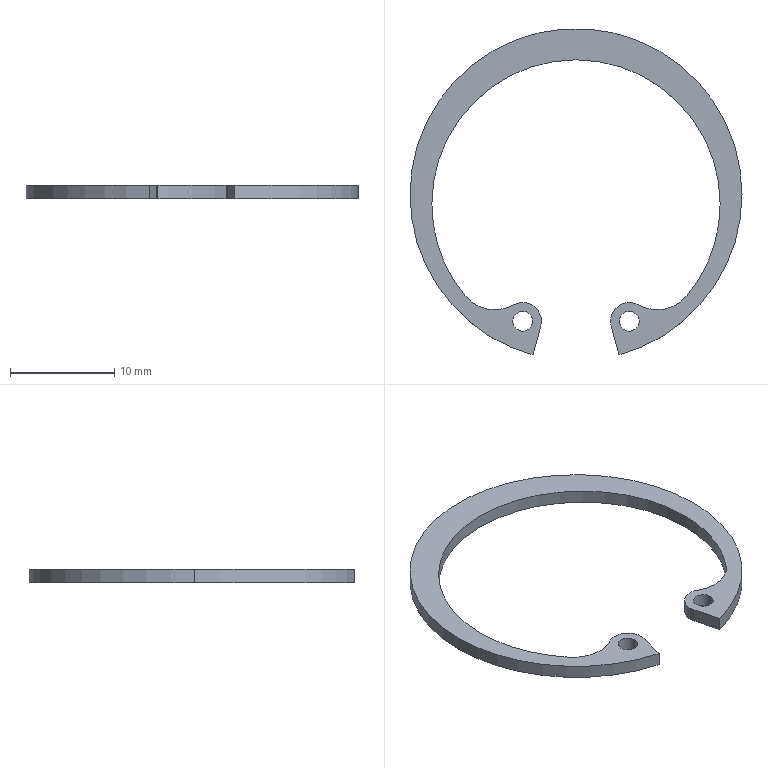Part | SolidWorks | features Extrusion 1 | 1 solid | 19 faces | box 31.9 x 31.357 x 1.3 mm | volume 270.021 mm3 | cylinder 15 | plane 4 | commonest cylinder face diameters 1.9 x4 3.6 x3 27.7 x3 31.9 x3 7.4 x2
STEP:
#1=CARTESIAN_POINT('',(-4.173,-11.265,1.3));
#2=VERTEX_POINT('',#1);
#3=CARTESIAN_POINT('',(-6.073,-11.265,1.3));
#4=VERTEX_POINT('',#3);
#5=CARTESIAN_POINT('',(-5.123,-11.265,1.3));
#6=DIRECTION('',(0.,0.,-1.));
#7=DIRECTION('',(1.,0.,0.));
#8=AXIS2_PLACEMENT_3D('',#5,#6,#7);
#9=CIRCLE('',#8,0.95);
#10=EDGE_CURVE('',#2,#4,#9,.T.);
#11=ORIENTED_EDGE('',*,*,#10,.F.);
#12=CARTESIAN_POINT('',(-4.173,-11.265,0.));
#13=VERTEX_POINT('',#12);
#14=CARTESIAN_POINT('',(-4.173,-11.265,1.3));
#15=DIRECTION('',(0.,0.,-1.));
#16=VECTOR('',#15,1000.);
#17=LINE('',#14,#16);
#18=EDGE_CURVE('',#2,#13,#17,.T.);
#19=ORIENTED_EDGE('',*,*,#18,.T.);
#20=CARTESIAN_POINT('',(-6.073,-11.265,0.));
#21=VERTEX_POINT('',#20);
#22=CARTESIAN_POINT('',(-5.123,-11.265,0.));
#23=DIRECTION('',(0.,0.,-1.));
#24=DIRECTION('',(1.,0.,0.));
#25=AXIS2_PLACEMENT_3D('',#22,#23,#24);
#26=CIRCLE('',#25,0.95);
#27=EDGE_CURVE('',#13,#21,#26,.T.);
#28=ORIENTED_EDGE('',*,*,#27,.T.);
#29=CARTESIAN_POINT('',(-6.073,-11.265,1.3));
#30=DIRECTION('',(0.,0.,-1.));
#31=VECTOR('',#30,1000.);
#32=LINE('',#29,#31);
#33=EDGE_CURVE('',#4,#21,#32,.T.);
#34=ORIENTED_EDGE('',*,*,#33,.F.);
#35=EDGE_LOOP('',(#11,#19,#28,#34));
#36=FACE_OUTER_BOUND('',#35,.T.);
#37=CARTESIAN_POINT('',(-5.123,-11.265,1.3));
#38=DIRECTION('',(0.,0.,-1.));
#39=DIRECTION('',(-1.,0.,0.));
#40=AXIS2_PLACEMENT_3D('',#37,#38,#39);
#41=CYLINDRICAL_SURFACE('',#40,0.95);
#42=ADVANCED_FACE('',(#36),#41,.F.);
#43=CARTESIAN_POINT('',(4.173,-11.265,1.3));
#44=VERTEX_POINT('',#43);
#45=CARTESIAN_POINT('',(6.073,-11.265,1.3));
#46=VERTEX_POINT('',#45);
#47=CARTESIAN_POINT('',(5.123,-11.265,1.3));
#48=DIRECTION('',(0.,0.,1.));
#49=DIRECTION('',(1.,0.,0.));
#50=AXIS2_PLACEMENT_3D('',#47,#48,#49);
#51=CIRCLE('',#50,0.95);
#52=EDGE_CURVE('',#44,#46,#51,.T.);
#53=ORIENTED_EDGE('',*,*,#52,.T.);
#54=CARTESIAN_POINT('',(6.073,-11.265,0.));
#55=VERTEX_POINT('',#54);
#56=CARTESIAN_POINT('',(6.073,-11.265,1.3));
#57=DIRECTION('',(0.,0.,-1.));
#58=VECTOR('',#57,1000.);
#59=LINE('',#56,#58);
#60=EDGE_CURVE('',#46,#55,#59,.T.);
#61=ORIENTED_EDGE('',*,*,#60,.T.);
#62=CARTESIAN_POINT('',(4.173,-11.265,0.));
#63=VERTEX_POINT('',#62);
#64=CARTESIAN_POINT('',(5.123,-11.265,0.));
#65=DIRECTION('',(0.,0.,1.));
#66=DIRECTION('',(1.,0.,0.));
#67=AXIS2_PLACEMENT_3D('',#64,#65,#66);
#68=CIRCLE('',#67,0.95);
#69=EDGE_CURVE('',#63,#55,#68,.T.);
#70=ORIENTED_EDGE('',*,*,#69,.F.);
#71=CARTESIAN_POINT('',(4.173,-11.265,1.3));
#72=DIRECTION('',(0.,0.,-1.));
#73=VECTOR('',#72,1000.);
#74=LINE('',#71,#73);
#75=EDGE_CURVE('',#44,#63,#74,.T.);
#76=ORIENTED_EDGE('',*,*,#75,.F.);
#77=EDGE_LOOP('',(#53,#61,#70,#76));
#78=FACE_OUTER_BOUND('',#77,.T.);
#79=CARTESIAN_POINT('',(5.123,-11.265,1.3));
#80=DIRECTION('',(0.,0.,-1.));
#81=DIRECTION('',(-1.,0.,0.));
#82=AXIS2_PLACEMENT_3D('',#79,#80,#81);
#83=CYLINDRICAL_SURFACE('',#82,0.95);
#84=ADVANCED_FACE('',(#78),#83,.F.);
#85=CARTESIAN_POINT('',(15.95,0.9,1.3));
#86=VERTEX_POINT('',#85);
#87=CARTESIAN_POINT('',(-15.95,0.9,1.3));
#88=VERTEX_POINT('',#87);
#89=CARTESIAN_POINT('',(0.,0.9,1.3));
#90=DIRECTION('',(0.,0.,1.));
#91=DIRECTION('',(1.,0.,0.));
#92=AXIS2_PLACEMENT_3D('',#89,#90,#91);
#93=CIRCLE('',#92,15.95);
#94=EDGE_CURVE('',#86,#88,#93,.T.);
#95=ORIENTED_EDGE('',*,*,#94,.F.);
#96=CARTESIAN_POINT('',(15.95,0.9,0.));
#97=VERTEX_POINT('',#96);
#98=CARTESIAN_POINT('',(15.95,0.9,1.3));
#99=DIRECTION('',(0.,0.,-1.));
#100=VECTOR('',#99,1000.);
#101=LINE('',#98,#100);
#102=EDGE_CURVE('',#86,#97,#101,.T.);
#103=ORIENTED_EDGE('',*,*,#102,.T.);
#104=CARTESIAN_POINT('',(-15.95,0.9,0.));
#105=VERTEX_POINT('',#104);
#106=CARTESIAN_POINT('',(0.,0.9,0.));
#107=DIRECTION('',(0.,0.,1.));
#108=DIRECTION('',(1.,0.,0.));
#109=AXIS2_PLACEMENT_3D('',#106,#107,#108);
#110=CIRCLE('',#109,15.95);
#111=EDGE_CURVE('',#97,#105,#110,.T.);
#112=ORIENTED_EDGE('',*,*,#111,.T.);
#113=CARTESIAN_POINT('',(-15.95,0.9,1.3));
#114=DIRECTION('',(0.,0.,-1.));
#115=VECTOR('',#114,1000.);
#116=LINE('',#113,#115);
#117=EDGE_CURVE('',#88,#105,#116,.T.);
#118=ORIENTED_EDGE('',*,*,#117,.F.);
#119=EDGE_LOOP('',(#95,#103,#112,#118));
#120=FACE_OUTER_BOUND('',#119,.T.);
#121=CARTESIAN_POINT('',(0.,0.9,1.3));
#122=DIRECTION('',(0.,0.,-1.));
#123=DIRECTION('',(-1.,0.,0.));
#124=AXIS2_PLACEMENT_3D('',#121,#122,#123);
#125=CYLINDRICAL_SURFACE('',#124,15.95);
#126=ADVANCED_FACE('',(#120),#125,.T.);
#127=CARTESIAN_POINT('',(-4.128,-14.507,1.3));
#128=VERTEX_POINT('',#127);
#129=CARTESIAN_POINT('',(0.,0.9,1.3));
#130=DIRECTION('',(0.,0.,1.));
#131=DIRECTION('',(1.,0.,0.));
#132=AXIS2_PLACEMENT_3D('',#129,#130,#131);
#133=CIRCLE('',#132,15.95);
#134=EDGE_CURVE('',#88,#128,#133,.T.);
#135=ORIENTED_EDGE('',*,*,#134,.F.);
#136=ORIENTED_EDGE('',*,*,#117,.T.);
#137=CARTESIAN_POINT('',(-4.128,-14.507,0.));
#138=VERTEX_POINT('',#137);
#139=CARTESIAN_POINT('',(0.,0.9,0.));
#140=DIRECTION('',(0.,0.,1.));
#141=DIRECTION('',(1.,0.,0.));
#142=AXIS2_PLACEMENT_3D('',#139,#140,#141);
#143=CIRCLE('',#142,15.95);
#144=EDGE_CURVE('',#105,#138,#143,.T.);
#145=ORIENTED_EDGE('',*,*,#144,.T.);
#146=CARTESIAN_POINT('',(-4.128,-14.507,1.3));
#147=DIRECTION('',(0.,0.,-1.));
#148=VECTOR('',#147,1000.);
#149=LINE('',#146,#148);
#150=EDGE_CURVE('',#128,#138,#149,.T.);
#151=ORIENTED_EDGE('',*,*,#150,.F.);
#152=EDGE_LOOP('',(#135,#136,#145,#151));
#153=FACE_OUTER_BOUND('',#152,.T.);
#154=CARTESIAN_POINT('',(0.,0.9,1.3));
#155=DIRECTION('',(0.,0.,-1.));
#156=DIRECTION('',(-1.,0.,0.));
#157=AXIS2_PLACEMENT_3D('',#154,#155,#156);
#158=CYLINDRICAL_SURFACE('',#157,15.95);
#159=ADVANCED_FACE('',(#153),#158,.T.);
#160=CARTESIAN_POINT('',(3.323,-11.265,1.3));
#161=VERTEX_POINT('',#160);
#162=CARTESIAN_POINT('',(3.384,-11.731,1.3));
#163=VERTEX_POINT('',#162);
#164=CARTESIAN_POINT('',(5.123,-11.265,1.3));
#165=DIRECTION('',(0.,0.,1.));
#166=DIRECTION('',(1.,0.,0.));
#167=AXIS2_PLACEMENT_3D('',#164,#165,#166);
#168=CIRCLE('',#167,1.8);
#169=EDGE_CURVE('',#161,#163,#168,.T.);
#170=ORIENTED_EDGE('',*,*,#169,.F.);
#171=CARTESIAN_POINT('',(3.323,-11.265,0.));
#172=VERTEX_POINT('',#171);
#173=CARTESIAN_POINT('',(3.323,-11.265,1.3));
#174=DIRECTION('',(0.,0.,-1.));
#175=VECTOR('',#174,1000.);
#176=LINE('',#173,#175);
#177=EDGE_CURVE('',#161,#172,#176,.T.);
#178=ORIENTED_EDGE('',*,*,#177,.T.);
#179=CARTESIAN_POINT('',(3.384,-11.731,0.));
#180=VERTEX_POINT('',#179);
#181=CARTESIAN_POINT('',(5.123,-11.265,0.));
#182=DIRECTION('',(0.,0.,1.));
#183=DIRECTION('',(1.,0.,0.));
#184=AXIS2_PLACEMENT_3D('',#181,#182,#183);
#185=CIRCLE('',#184,1.8);
#186=EDGE_CURVE('',#172,#180,#185,.T.);
#187=ORIENTED_EDGE('',*,*,#186,.T.);
#188=CARTESIAN_POINT('',(3.384,-11.731,1.3));
#189=DIRECTION('',(0.,0.,-1.));
#190=VECTOR('',#189,1000.);
#191=LINE('',#188,#190);
#192=EDGE_CURVE('',#163,#180,#191,.T.);
#193=ORIENTED_EDGE('',*,*,#192,.F.);
#194=EDGE_LOOP('',(#170,#178,#187,#193));
#195=FACE_OUTER_BOUND('',#194,.T.);
#196=CARTESIAN_POINT('',(5.123,-11.265,1.3));
#197=DIRECTION('',(0.,0.,-1.));
#198=DIRECTION('',(-1.,0.,0.));
#199=AXIS2_PLACEMENT_3D('',#196,#197,#198);
#200=CYLINDRICAL_SURFACE('',#199,1.8);
#201=ADVANCED_FACE('',(#195),#200,.T.);
#202=CARTESIAN_POINT('',(10.67,-8.831,1.3));
#203=VERTEX_POINT('',#202);
#204=CARTESIAN_POINT('',(13.85,0.,1.3));
#205=VERTEX_POINT('',#204);
#206=CARTESIAN_POINT('',(0.,0.,1.3));
#207=DIRECTION('',(0.,0.,1.));
#208=DIRECTION('',(1.,0.,0.));
#209=AXIS2_PLACEMENT_3D('',#206,#207,#208);
#210=CIRCLE('',#209,13.85);
#211=EDGE_CURVE('',#203,#205,#210,.T.);
#212=ORIENTED_EDGE('',*,*,#211,.T.);
#213=CARTESIAN_POINT('',(13.85,0.,0.));
#214=VERTEX_POINT('',#213);
#215=CARTESIAN_POINT('',(13.85,0.,1.3));
#216=DIRECTION('',(0.,0.,-1.));
#217=VECTOR('',#216,1000.);
#218=LINE('',#215,#217);
#219=EDGE_CURVE('',#205,#214,#218,.T.);
#220=ORIENTED_EDGE('',*,*,#219,.T.);
#221=CARTESIAN_POINT('',(10.67,-8.831,0.));
#222=VERTEX_POINT('',#221);
#223=CARTESIAN_POINT('',(0.,0.,0.));
#224=DIRECTION('',(0.,0.,1.));
#225=DIRECTION('',(1.,0.,0.));
#226=AXIS2_PLACEMENT_3D('',#223,#224,#225);
#227=CIRCLE('',#226,13.85);
#228=EDGE_CURVE('',#222,#214,#227,.T.);
#229=ORIENTED_EDGE('',*,*,#228,.F.);
#230=CARTESIAN_POINT('',(10.67,-8.831,1.3));
#231=DIRECTION('',(0.,0.,-1.));
#232=VECTOR('',#231,1000.);
#233=LINE('',#230,#232);
#234=EDGE_CURVE('',#203,#222,#233,.T.);
#235=ORIENTED_EDGE('',*,*,#234,.F.);
#236=EDGE_LOOP('',(#212,#220,#229,#235));
#237=FACE_OUTER_BOUND('',#236,.T.);
#238=CARTESIAN_POINT('',(0.,0.,1.3));
#239=DIRECTION('',(0.,0.,-1.));
#240=DIRECTION('',(-1.,0.,0.));
#241=AXIS2_PLACEMENT_3D('',#238,#239,#240);
#242=CYLINDRICAL_SURFACE('',#241,13.85);
#243=ADVANCED_FACE('',(#237),#242,.F.);
#244=ORIENTED_EDGE('',*,*,#219,.F.);
#245=CARTESIAN_POINT('',(-13.85,0.,1.3));
#246=VERTEX_POINT('',#245);
#247=CARTESIAN_POINT('',(0.,0.,1.3));
#248=DIRECTION('',(0.,0.,1.));
#249=DIRECTION('',(1.,0.,0.));
#250=AXIS2_PLACEMENT_3D('',#247,#248,#249);
#251=CIRCLE('',#250,13.85);
#252=EDGE_CURVE('',#205,#246,#251,.T.);
#253=ORIENTED_EDGE('',*,*,#252,.T.);
#254=CARTESIAN_POINT('',(-13.85,0.,0.));
#255=VERTEX_POINT('',#254);
#256=CARTESIAN_POINT('',(-13.85,0.,1.3));
#257=DIRECTION('',(0.,0.,-1.));
#258=VECTOR('',#257,1000.);
#259=LINE('',#256,#258);
#260=EDGE_CURVE('',#246,#255,#259,.T.);
#261=ORIENTED_EDGE('',*,*,#260,.T.);
#262=CARTESIAN_POINT('',(0.,0.,0.));
#263=DIRECTION('',(0.,0.,1.));
#264=DIRECTION('',(1.,0.,0.));
#265=AXIS2_PLACEMENT_3D('',#262,#263,#264);
#266=CIRCLE('',#265,13.85);
#267=EDGE_CURVE('',#214,#255,#266,.T.);
#268=ORIENTED_EDGE('',*,*,#267,.F.);
#269=EDGE_LOOP('',(#244,#253,#261,#268));
#270=FACE_OUTER_BOUND('',#269,.T.);
#271=CARTESIAN_POINT('',(0.,0.,1.3));
#272=DIRECTION('',(0.,0.,-1.));
#273=DIRECTION('',(-1.,0.,0.));
#274=AXIS2_PLACEMENT_3D('',#271,#272,#273);
#275=CYLINDRICAL_SURFACE('',#274,13.85);
#276=ADVANCED_FACE('',(#270),#275,.F.);
#277=CARTESIAN_POINT('',(-6.006,-9.696,0.));
#278=VERTEX_POINT('',#277);
#279=CARTESIAN_POINT('',(-3.384,-11.731,0.));
#280=VERTEX_POINT('',#279);
#281=CARTESIAN_POINT('',(-5.123,-11.265,0.));
#282=DIRECTION('',(0.,0.,-1.));
#283=DIRECTION('',(1.,0.,0.));
#284=AXIS2_PLACEMENT_3D('',#281,#282,#283);
#285=CIRCLE('',#284,1.8);
#286=EDGE_CURVE('',#278,#280,#285,.T.);
#287=ORIENTED_EDGE('',*,*,#286,.F.);
#288=CARTESIAN_POINT('',(-6.006,-9.696,1.3));
#289=VERTEX_POINT('',#288);
#290=CARTESIAN_POINT('',(-6.006,-9.696,1.3));
#291=DIRECTION('',(0.,0.,-1.));
#292=VECTOR('',#291,1000.);
#293=LINE('',#290,#292);
#294=EDGE_CURVE('',#289,#278,#293,.T.);
#295=ORIENTED_EDGE('',*,*,#294,.F.);
#296=CARTESIAN_POINT('',(-3.384,-11.731,1.3));
#297=VERTEX_POINT('',#296);
#298=CARTESIAN_POINT('',(-5.123,-11.265,1.3));
#299=DIRECTION('',(0.,0.,-1.));
#300=DIRECTION('',(1.,0.,0.));
#301=AXIS2_PLACEMENT_3D('',#298,#299,#300);
#302=CIRCLE('',#301,1.8);
#303=EDGE_CURVE('',#289,#297,#302,.T.);
#304=ORIENTED_EDGE('',*,*,#303,.T.);
#305=CARTESIAN_POINT('',(-3.384,-11.731,1.3));
#306=DIRECTION('',(0.,0.,-1.));
#307=VECTOR('',#306,1000.);
#308=LINE('',#305,#307);
#309=EDGE_CURVE('',#297,#280,#308,.T.);
#310=ORIENTED_EDGE('',*,*,#309,.T.);
#311=EDGE_LOOP('',(#287,#295,#304,#310));
#312=FACE_OUTER_BOUND('',#311,.T.);
#313=CARTESIAN_POINT('',(-5.123,-11.265,1.3));
#314=DIRECTION('',(0.,0.,-1.));
#315=DIRECTION('',(-1.,0.,0.));
#316=AXIS2_PLACEMENT_3D('',#313,#314,#315);
#317=CYLINDRICAL_SURFACE('',#316,1.8);
#318=ADVANCED_FACE('',(#312),#317,.T.);
#319=CARTESIAN_POINT('',(-10.67,-8.831,0.));
#320=VERTEX_POINT('',#319);
#321=CARTESIAN_POINT('',(-7.819,-6.471,0.));
#322=DIRECTION('',(0.,0.,-1.));
#323=DIRECTION('',(1.,0.,0.));
#324=AXIS2_PLACEMENT_3D('',#321,#322,#323);
#325=CIRCLE('',#324,3.7);
#326=EDGE_CURVE('',#278,#320,#325,.T.);
#327=ORIENTED_EDGE('',*,*,#326,.T.);
#328=CARTESIAN_POINT('',(-10.67,-8.831,1.3));
#329=VERTEX_POINT('',#328);
#330=CARTESIAN_POINT('',(-10.67,-8.831,1.3));
#331=DIRECTION('',(0.,0.,-1.));
#332=VECTOR('',#331,1000.);
#333=LINE('',#330,#332);
#334=EDGE_CURVE('',#329,#320,#333,.T.);
#335=ORIENTED_EDGE('',*,*,#334,.F.);
#336=CARTESIAN_POINT('',(-7.819,-6.471,1.3));
#337=DIRECTION('',(0.,0.,-1.));
#338=DIRECTION('',(1.,0.,0.));
#339=AXIS2_PLACEMENT_3D('',#336,#337,#338);
#340=CIRCLE('',#339,3.7);
#341=EDGE_CURVE('',#289,#329,#340,.T.);
#342=ORIENTED_EDGE('',*,*,#341,.F.);
#343=ORIENTED_EDGE('',*,*,#294,.T.);
#344=EDGE_LOOP('',(#327,#335,#342,#343));
#345=FACE_OUTER_BOUND('',#344,.T.);
#346=CARTESIAN_POINT('',(-7.819,-6.471,1.3));
#347=DIRECTION('',(0.,0.,-1.));
#348=DIRECTION('',(-1.,0.,0.));
#349=AXIS2_PLACEMENT_3D('',#346,#347,#348);
#350=CYLINDRICAL_SURFACE('',#349,3.7);
#351=ADVANCED_FACE('',(#345),#350,.F.);
#352=ORIENTED_EDGE('',*,*,#260,.F.);
#353=CARTESIAN_POINT('',(0.,0.,1.3));
#354=DIRECTION('',(0.,0.,1.));
#355=DIRECTION('',(1.,0.,0.));
#356=AXIS2_PLACEMENT_3D('',#353,#354,#355);
#357=CIRCLE('',#356,13.85);
#358=EDGE_CURVE('',#246,#329,#357,.T.);
#359=ORIENTED_EDGE('',*,*,#358,.T.);
#360=ORIENTED_EDGE('',*,*,#334,.T.);
#361=CARTESIAN_POINT('',(0.,0.,0.));
#362=DIRECTION('',(0.,0.,1.));
#363=DIRECTION('',(1.,0.,0.));
#364=AXIS2_PLACEMENT_3D('',#361,#362,#363);
#365=CIRCLE('',#364,13.85);
#366=EDGE_CURVE('',#255,#320,#365,.T.);
#367=ORIENTED_EDGE('',*,*,#366,.F.);
#368=EDGE_LOOP('',(#352,#359,#360,#367));
#369=FACE_OUTER_BOUND('',#368,.T.);
#370=CARTESIAN_POINT('',(0.,0.,1.3));
#371=DIRECTION('',(0.,0.,-1.));
#372=DIRECTION('',(-1.,0.,0.));
#373=AXIS2_PLACEMENT_3D('',#370,#371,#372);
#374=CYLINDRICAL_SURFACE('',#373,13.85);
#375=ADVANCED_FACE('',(#369),#374,.F.);
#376=CARTESIAN_POINT('',(6.006,-9.696,0.));
#377=VERTEX_POINT('',#376);
#378=CARTESIAN_POINT('',(7.819,-6.471,0.));
#379=DIRECTION('',(0.,0.,1.));
#380=DIRECTION('',(1.,0.,0.));
#381=AXIS2_PLACEMENT_3D('',#378,#379,#380);
#382=CIRCLE('',#381,3.7);
#383=EDGE_CURVE('',#377,#222,#382,.T.);
#384=ORIENTED_EDGE('',*,*,#383,.F.);
#385=CARTESIAN_POINT('',(6.006,-9.696,1.3));
#386=VERTEX_POINT('',#385);
#387=CARTESIAN_POINT('',(6.006,-9.696,1.3));
#388=DIRECTION('',(0.,0.,-1.));
#389=VECTOR('',#388,1000.);
#390=LINE('',#387,#389);
#391=EDGE_CURVE('',#386,#377,#390,.T.);
#392=ORIENTED_EDGE('',*,*,#391,.F.);
#393=CARTESIAN_POINT('',(7.819,-6.471,1.3));
#394=DIRECTION('',(0.,0.,1.));
#395=DIRECTION('',(1.,0.,0.));
#396=AXIS2_PLACEMENT_3D('',#393,#394,#395);
#397=CIRCLE('',#396,3.7);
#398=EDGE_CURVE('',#386,#203,#397,.T.);
#399=ORIENTED_EDGE('',*,*,#398,.T.);
#400=ORIENTED_EDGE('',*,*,#234,.T.);
#401=EDGE_LOOP('',(#384,#392,#399,#400));
#402=FACE_OUTER_BOUND('',#401,.T.);
#403=CARTESIAN_POINT('',(7.819,-6.471,1.3));
#404=DIRECTION('',(0.,0.,-1.));
#405=DIRECTION('',(-1.,0.,0.));
#406=AXIS2_PLACEMENT_3D('',#403,#404,#405);
#407=CYLINDRICAL_SURFACE('',#406,3.7);
#408=ADVANCED_FACE('',(#402),#407,.F.);
#409=ORIENTED_EDGE('',*,*,#177,.F.);
#410=CARTESIAN_POINT('',(5.123,-11.265,1.3));
#411=DIRECTION('',(0.,0.,1.));
#412=DIRECTION('',(1.,0.,0.));
#413=AXIS2_PLACEMENT_3D('',#410,#411,#412);
#414=CIRCLE('',#413,1.8);
#415=EDGE_CURVE('',#386,#161,#414,.T.);
#416=ORIENTED_EDGE('',*,*,#415,.F.);
#417=ORIENTED_EDGE('',*,*,#391,.T.);
#418=CARTESIAN_POINT('',(5.123,-11.265,0.));
#419=DIRECTION('',(0.,0.,1.));
#420=DIRECTION('',(1.,0.,0.));
#421=AXIS2_PLACEMENT_3D('',#418,#419,#420);
#422=CIRCLE('',#421,1.8);
#423=EDGE_CURVE('',#377,#172,#422,.T.);
#424=ORIENTED_EDGE('',*,*,#423,.T.);
#425=EDGE_LOOP('',(#409,#416,#417,#424));
#426=FACE_OUTER_BOUND('',#425,.T.);
#427=CARTESIAN_POINT('',(5.123,-11.265,1.3));
#428=DIRECTION('',(0.,0.,-1.));
#429=DIRECTION('',(-1.,0.,0.));
#430=AXIS2_PLACEMENT_3D('',#427,#428,#429);
#431=CYLINDRICAL_SURFACE('',#430,1.8);
#432=ADVANCED_FACE('',(#426),#431,.T.);
#433=CARTESIAN_POINT('',(4.128,-14.507,0.));
#434=VERTEX_POINT('',#433);
#435=CARTESIAN_POINT('',(0.225,0.06029,0.));
#436=DIRECTION('',(0.2588,-0.9659,0.));
#437=VECTOR('',#436,1000.);
#438=LINE('',#435,#437);
#439=EDGE_CURVE('',#180,#434,#438,.T.);
#440=ORIENTED_EDGE('',*,*,#439,.T.);
#441=CARTESIAN_POINT('',(4.128,-14.507,1.3));
#442=VERTEX_POINT('',#441);
#443=CARTESIAN_POINT('',(4.128,-14.507,1.3));
#444=DIRECTION('',(0.,0.,-1.));
#445=VECTOR('',#444,1000.);
#446=LINE('',#443,#445);
#447=EDGE_CURVE('',#442,#434,#446,.T.);
#448=ORIENTED_EDGE('',*,*,#447,.F.);
#449=CARTESIAN_POINT('',(0.225,0.06029,1.3));
#450=DIRECTION('',(0.2588,-0.9659,0.));
#451=VECTOR('',#450,1000.);
#452=LINE('',#449,#451);
#453=EDGE_CURVE('',#163,#442,#452,.T.);
#454=ORIENTED_EDGE('',*,*,#453,.F.);
#455=ORIENTED_EDGE('',*,*,#192,.T.);
#456=EDGE_LOOP('',(#440,#448,#454,#455));
#457=FACE_OUTER_BOUND('',#456,.T.);
#458=CARTESIAN_POINT('',(0.225,0.06029,1.3));
#459=DIRECTION('',(0.9659,0.2588,0.));
#460=DIRECTION('',(-0.2588,0.9659,0.));
#461=AXIS2_PLACEMENT_3D('',#458,#459,#460);
#462=PLANE('',#461);
#463=ADVANCED_FACE('',(#457),#462,.F.);
#464=ORIENTED_EDGE('',*,*,#102,.F.);
#465=CARTESIAN_POINT('',(0.,0.9,1.3));
#466=DIRECTION('',(0.,0.,1.));
#467=DIRECTION('',(1.,0.,0.));
#468=AXIS2_PLACEMENT_3D('',#465,#466,#467);
#469=CIRCLE('',#468,15.95);
#470=EDGE_CURVE('',#442,#86,#469,.T.);
#471=ORIENTED_EDGE('',*,*,#470,.F.);
#472=ORIENTED_EDGE('',*,*,#447,.T.);
#473=CARTESIAN_POINT('',(0.,0.9,0.));
#474=DIRECTION('',(0.,0.,1.));
#475=DIRECTION('',(1.,0.,0.));
#476=AXIS2_PLACEMENT_3D('',#473,#474,#475);
#477=CIRCLE('',#476,15.95);
#478=EDGE_CURVE('',#434,#97,#477,.T.);
#479=ORIENTED_EDGE('',*,*,#478,.T.);
#480=EDGE_LOOP('',(#464,#471,#472,#479));
#481=FACE_OUTER_BOUND('',#480,.T.);
#482=CARTESIAN_POINT('',(0.,0.9,1.3));
#483=DIRECTION('',(0.,0.,-1.));
#484=DIRECTION('',(-1.,0.,0.));
#485=AXIS2_PLACEMENT_3D('',#482,#483,#484);
#486=CYLINDRICAL_SURFACE('',#485,15.95);
#487=ADVANCED_FACE('',(#481),#486,.T.);
#488=ORIENTED_EDGE('',*,*,#60,.F.);
#489=CARTESIAN_POINT('',(5.123,-11.265,1.3));
#490=DIRECTION('',(0.,0.,1.));
#491=DIRECTION('',(1.,0.,0.));
#492=AXIS2_PLACEMENT_3D('',#489,#490,#491);
#493=CIRCLE('',#492,0.95);
#494=EDGE_CURVE('',#46,#44,#493,.T.);
#495=ORIENTED_EDGE('',*,*,#494,.T.);
#496=ORIENTED_EDGE('',*,*,#75,.T.);
#497=CARTESIAN_POINT('',(5.123,-11.265,0.));
#498=DIRECTION('',(0.,0.,1.));
#499=DIRECTION('',(1.,0.,0.));
#500=AXIS2_PLACEMENT_3D('',#497,#498,#499);
#501=CIRCLE('',#500,0.95);
#502=EDGE_CURVE('',#55,#63,#501,.T.);
#503=ORIENTED_EDGE('',*,*,#502,.F.);
#504=EDGE_LOOP('',(#488,#495,#496,#503));
#505=FACE_OUTER_BOUND('',#504,.T.);
#506=CARTESIAN_POINT('',(5.123,-11.265,1.3));
#507=DIRECTION('',(0.,0.,-1.));
#508=DIRECTION('',(-1.,0.,0.));
#509=AXIS2_PLACEMENT_3D('',#506,#507,#508);
#510=CYLINDRICAL_SURFACE('',#509,0.95);
#511=ADVANCED_FACE('',(#505),#510,.F.);
#512=CARTESIAN_POINT('',(-0.225,0.06029,0.));
#513=DIRECTION('',(-0.2588,-0.9659,0.));
#514=VECTOR('',#513,1000.);
#515=LINE('',#512,#514);
#516=EDGE_CURVE('',#280,#138,#515,.T.);
#517=ORIENTED_EDGE('',*,*,#516,.F.);
#518=ORIENTED_EDGE('',*,*,#309,.F.);
#519=CARTESIAN_POINT('',(-0.225,0.06029,1.3));
#520=DIRECTION('',(-0.2588,-0.9659,0.));
#521=VECTOR('',#520,1000.);
#522=LINE('',#519,#521);
#523=EDGE_CURVE('',#297,#128,#522,.T.);
#524=ORIENTED_EDGE('',*,*,#523,.T.);
#525=ORIENTED_EDGE('',*,*,#150,.T.);
#526=EDGE_LOOP('',(#517,#518,#524,#525));
#527=FACE_OUTER_BOUND('',#526,.T.);
#528=CARTESIAN_POINT('',(-0.225,0.06029,1.3));
#529=DIRECTION('',(0.9659,-0.2588,0.));
#530=DIRECTION('',(0.2588,0.9659,0.));
#531=AXIS2_PLACEMENT_3D('',#528,#529,#530);
#532=PLANE('',#531);
#533=ADVANCED_FACE('',(#527),#532,.T.);
#534=ORIENTED_EDGE('',*,*,#18,.F.);
#535=CARTESIAN_POINT('',(-5.123,-11.265,1.3));
#536=DIRECTION('',(0.,0.,-1.));
#537=DIRECTION('',(1.,0.,0.));
#538=AXIS2_PLACEMENT_3D('',#535,#536,#537);
#539=CIRCLE('',#538,0.95);
#540=EDGE_CURVE('',#4,#2,#539,.T.);
#541=ORIENTED_EDGE('',*,*,#540,.F.);
#542=ORIENTED_EDGE('',*,*,#33,.T.);
#543=CARTESIAN_POINT('',(-5.123,-11.265,0.));
#544=DIRECTION('',(0.,0.,-1.));
#545=DIRECTION('',(1.,0.,0.));
#546=AXIS2_PLACEMENT_3D('',#543,#544,#545);
#547=CIRCLE('',#546,0.95);
#548=EDGE_CURVE('',#21,#13,#547,.T.);
#549=ORIENTED_EDGE('',*,*,#548,.T.);
#550=EDGE_LOOP('',(#534,#541,#542,#549));
#551=FACE_OUTER_BOUND('',#550,.T.);
#552=CARTESIAN_POINT('',(-5.123,-11.265,1.3));
#553=DIRECTION('',(0.,0.,-1.));
#554=DIRECTION('',(-1.,0.,0.));
#555=AXIS2_PLACEMENT_3D('',#552,#553,#554);
#556=CYLINDRICAL_SURFACE('',#555,0.95);
#557=ADVANCED_FACE('',(#551),#556,.F.);
#558=ORIENTED_EDGE('',*,*,#303,.F.);
#559=ORIENTED_EDGE('',*,*,#341,.T.);
#560=ORIENTED_EDGE('',*,*,#358,.F.);
#561=ORIENTED_EDGE('',*,*,#252,.F.);
#562=ORIENTED_EDGE('',*,*,#211,.F.);
#563=ORIENTED_EDGE('',*,*,#398,.F.);
#564=ORIENTED_EDGE('',*,*,#415,.T.);
#565=ORIENTED_EDGE('',*,*,#169,.T.);
#566=ORIENTED_EDGE('',*,*,#453,.T.);
#567=ORIENTED_EDGE('',*,*,#470,.T.);
#568=ORIENTED_EDGE('',*,*,#94,.T.);
#569=ORIENTED_EDGE('',*,*,#134,.T.);
#570=ORIENTED_EDGE('',*,*,#523,.F.);
#571=EDGE_LOOP('',(#558,#559,#560,#561,#562,#563,#564,#565,#566,#567,#568,#569,#570));
#572=FACE_OUTER_BOUND('',#571,.T.);
#573=ORIENTED_EDGE('',*,*,#52,.F.);
#574=ORIENTED_EDGE('',*,*,#494,.F.);
#575=EDGE_LOOP('',(#573,#574));
#576=FACE_BOUND('',#575,.T.);
#577=ORIENTED_EDGE('',*,*,#540,.T.);
#578=ORIENTED_EDGE('',*,*,#10,.T.);
#579=EDGE_LOOP('',(#577,#578));
#580=FACE_BOUND('',#579,.T.);
#581=CARTESIAN_POINT('',(0.,0.,1.3));
#582=DIRECTION('',(0.,0.,1.));
#583=DIRECTION('',(1.,0.,0.));
#584=AXIS2_PLACEMENT_3D('',#581,#582,#583);
#585=PLANE('',#584);
#586=ADVANCED_FACE('',(#572,#576,#580),#585,.T.);
#587=ORIENTED_EDGE('',*,*,#286,.T.);
#588=ORIENTED_EDGE('',*,*,#516,.T.);
#589=ORIENTED_EDGE('',*,*,#144,.F.);
#590=ORIENTED_EDGE('',*,*,#111,.F.);
#591=ORIENTED_EDGE('',*,*,#478,.F.);
#592=ORIENTED_EDGE('',*,*,#439,.F.);
#593=ORIENTED_EDGE('',*,*,#186,.F.);
#594=ORIENTED_EDGE('',*,*,#423,.F.);
#595=ORIENTED_EDGE('',*,*,#383,.T.);
#596=ORIENTED_EDGE('',*,*,#228,.T.);
#597=ORIENTED_EDGE('',*,*,#267,.T.);
#598=ORIENTED_EDGE('',*,*,#366,.T.);
#599=ORIENTED_EDGE('',*,*,#326,.F.);
#600=EDGE_LOOP('',(#587,#588,#589,#590,#591,#592,#593,#594,#595,#596,#597,#598,#599));
#601=FACE_OUTER_BOUND('',#600,.T.);
#602=ORIENTED_EDGE('',*,*,#69,.T.);
#603=ORIENTED_EDGE('',*,*,#502,.T.);
#604=EDGE_LOOP('',(#602,#603));
#605=FACE_BOUND('',#604,.T.);
#606=ORIENTED_EDGE('',*,*,#548,.F.);
#607=ORIENTED_EDGE('',*,*,#27,.F.);
#608=EDGE_LOOP('',(#606,#607));
#609=FACE_BOUND('',#608,.T.);
#610=CARTESIAN_POINT('',(0.,0.,0.));
#611=DIRECTION('',(0.,0.,1.));
#612=DIRECTION('',(1.,0.,0.));
#613=AXIS2_PLACEMENT_3D('',#610,#611,#612);
#614=PLANE('',#613);
#615=ADVANCED_FACE('',(#601,#605,#609),#614,.F.);
#616=CLOSED_SHELL('',(#42,#84,#126,#159,#201,#243,#276,#318,#351,#375,#408,#432,#463,#487,#511,#533,#557,#586,#615));
#617=MANIFOLD_SOLID_BREP('',#616);
#618=CARTESIAN_POINT('',(0.,0.,0.));
#619=DIRECTION('',(0.,0.,1.));
#620=DIRECTION('',(1.,0.,0.));
#621=AXIS2_PLACEMENT_3D('',#618,#619,#620);
#622=(LENGTH_UNIT()NAMED_UNIT(*)SI_UNIT(.MILLI.,.METRE.));
#623=UNCERTAINTY_MEASURE_WITH_UNIT(LENGTH_MEASURE(0.00001),#622,'','');
#624=(NAMED_UNIT(*)PLANE_ANGLE_UNIT()SI_UNIT($,.RADIAN.));
#625=(NAMED_UNIT(*)SI_UNIT($,.STERADIAN.)SOLID_ANGLE_UNIT());
#626=(GEOMETRIC_REPRESENTATION_CONTEXT(3)GLOBAL_UNCERTAINTY_ASSIGNED_CONTEXT((#623))GLOBAL_UNIT_ASSIGNED_CONTEXT((#622,#624,#625))REPRESENTATION_CONTEXT('',''));
#627=ADVANCED_BREP_SHAPE_REPRESENTATION('',(#617,#621),#626);